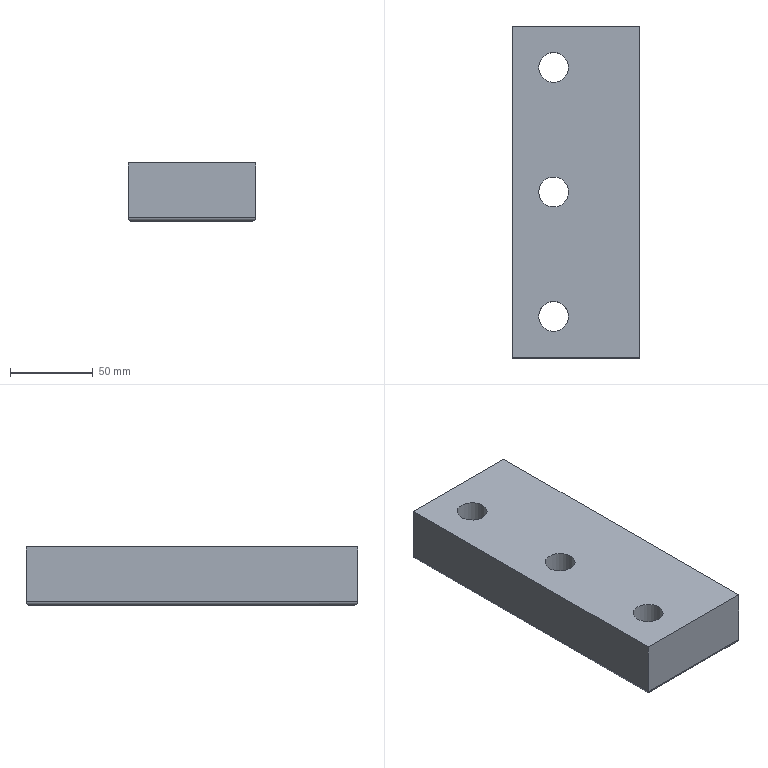Part | NX | features solid 2 | 1 solid | 13 faces | box 77 x 200 x 35 mm | volume 511808 mm3 | cylinder 7 | plane 6 | commonest cylinder face diameters 4 x4 18 x3
STEP:
#1=CARTESIAN_POINT('',(-648.,-745.,177.));
#2=VERTEX_POINT('',#1);
#3=CARTESIAN_POINT('',(-648.,-745.,210.));
#4=VERTEX_POINT('',#3);
#5=CARTESIAN_POINT('',(-648.,-745.,357.029));
#6=DIRECTION('',(0.,0.,-1.));
#7=VECTOR('',#6,1000.);
#8=LINE('',#5,#7);
#9=EDGE_CURVE('',#2,#4,#8,.F.);
#10=ORIENTED_EDGE('',*,*,#9,.F.);
#11=CARTESIAN_POINT('',(-648.,-545.,177.));
#12=VERTEX_POINT('',#11);
#13=CARTESIAN_POINT('',(-648.,-545.,177.));
#14=DIRECTION('',(0.,1.,0.));
#15=VECTOR('',#14,1000.);
#16=LINE('',#13,#15);
#17=EDGE_CURVE('',#2,#12,#16,.T.);
#18=ORIENTED_EDGE('',*,*,#17,.T.);
#19=CARTESIAN_POINT('',(-648.,-545.,210.));
#20=VERTEX_POINT('',#19);
#21=CARTESIAN_POINT('',(-648.,-545.,210.));
#22=DIRECTION('',(0.,0.,-1.));
#23=VECTOR('',#22,1000.);
#24=LINE('',#21,#23);
#25=EDGE_CURVE('',#12,#20,#24,.F.);
#26=ORIENTED_EDGE('',*,*,#25,.T.);
#27=CARTESIAN_POINT('',(-648.,-905.,210.));
#28=DIRECTION('',(0.,1.,0.));
#29=VECTOR('',#28,1000.);
#30=LINE('',#27,#29);
#31=EDGE_CURVE('',#4,#20,#30,.T.);
#32=ORIENTED_EDGE('',*,*,#31,.F.);
#33=EDGE_LOOP('',(#10,#18,#26,#32));
#34=FACE_BOUND('',#33,.T.);
#35=CARTESIAN_POINT('',(-648.,-905.,210.));
#36=DIRECTION('',(1.,0.,0.));
#37=DIRECTION('',(0.,1.,0.));
#38=AXIS2_PLACEMENT_3D('',#35,#36,#37);
#39=PLANE('',#38);
#40=ADVANCED_FACE('',(#34),#39,.T.);
#41=ORIENTED_EDGE('',*,*,#25,.F.);
#42=CARTESIAN_POINT('',(-725.,-545.,177.));
#43=VERTEX_POINT('',#42);
#44=CARTESIAN_POINT('',(-727.,-545.,177.));
#45=DIRECTION('',(-1.,0.,0.));
#46=VECTOR('',#45,1000.);
#47=LINE('',#44,#46);
#48=EDGE_CURVE('',#12,#43,#47,.T.);
#49=ORIENTED_EDGE('',*,*,#48,.T.);
#50=CARTESIAN_POINT('',(-725.,-545.,210.));
#51=VERTEX_POINT('',#50);
#52=CARTESIAN_POINT('',(-725.,-545.,268.));
#53=DIRECTION('',(0.,0.,1.));
#54=VECTOR('',#53,1000.);
#55=LINE('',#52,#54);
#56=EDGE_CURVE('',#43,#51,#55,.T.);
#57=ORIENTED_EDGE('',*,*,#56,.T.);
#58=CARTESIAN_POINT('',(-648.,-545.,210.));
#59=DIRECTION('',(1.,0.,0.));
#60=VECTOR('',#59,1000.);
#61=LINE('',#58,#60);
#62=EDGE_CURVE('',#20,#51,#61,.F.);
#63=ORIENTED_EDGE('',*,*,#62,.F.);
#64=EDGE_LOOP('',(#41,#49,#57,#63));
#65=FACE_BOUND('',#64,.T.);
#66=CARTESIAN_POINT('',(-671.,-545.,268.));
#67=DIRECTION('',(0.,-1.,0.));
#68=DIRECTION('',(1.,0.,0.));
#69=AXIS2_PLACEMENT_3D('',#66,#67,#68);
#70=PLANE('',#69);
#71=ADVANCED_FACE('',(#65),#70,.F.);
#72=ORIENTED_EDGE('',*,*,#56,.F.);
#73=CARTESIAN_POINT('',(-725.,-745.,177.));
#74=VERTEX_POINT('',#73);
#75=CARTESIAN_POINT('',(-725.,-745.,177.));
#76=DIRECTION('',(0.,1.,0.));
#77=VECTOR('',#76,1000.);
#78=LINE('',#75,#77);
#79=EDGE_CURVE('',#43,#74,#78,.F.);
#80=ORIENTED_EDGE('',*,*,#79,.T.);
#81=CARTESIAN_POINT('',(-725.,-745.,210.));
#82=VERTEX_POINT('',#81);
#83=CARTESIAN_POINT('',(-725.,-745.,210.));
#84=DIRECTION('',(0.,0.,1.));
#85=VECTOR('',#84,1000.);
#86=LINE('',#83,#85);
#87=EDGE_CURVE('',#74,#82,#86,.T.);
#88=ORIENTED_EDGE('',*,*,#87,.T.);
#89=CARTESIAN_POINT('',(-725.,-905.,210.));
#90=DIRECTION('',(0.,-1.,0.));
#91=VECTOR('',#90,1000.);
#92=LINE('',#89,#91);
#93=EDGE_CURVE('',#82,#51,#92,.F.);
#94=ORIENTED_EDGE('',*,*,#93,.T.);
#95=EDGE_LOOP('',(#72,#80,#88,#94));
#96=FACE_BOUND('',#95,.T.);
#97=CARTESIAN_POINT('',(-725.,-905.,210.));
#98=DIRECTION('',(1.,0.,0.));
#99=DIRECTION('',(0.,1.,0.));
#100=AXIS2_PLACEMENT_3D('',#97,#98,#99);
#101=PLANE('',#100);
#102=ADVANCED_FACE('',(#96),#101,.F.);
#103=ORIENTED_EDGE('',*,*,#87,.F.);
#104=CARTESIAN_POINT('',(-648.,-745.,177.));
#105=DIRECTION('',(-1.,0.,0.));
#106=VECTOR('',#105,1000.);
#107=LINE('',#104,#106);
#108=EDGE_CURVE('',#74,#2,#107,.F.);
#109=ORIENTED_EDGE('',*,*,#108,.T.);
#110=ORIENTED_EDGE('',*,*,#9,.T.);
#111=CARTESIAN_POINT('',(-71.,-745.,210.));
#112=DIRECTION('',(1.,0.,0.));
#113=VECTOR('',#112,1000.);
#114=LINE('',#111,#113);
#115=EDGE_CURVE('',#4,#82,#114,.F.);
#116=ORIENTED_EDGE('',*,*,#115,.T.);
#117=EDGE_LOOP('',(#103,#109,#110,#116));
#118=FACE_BOUND('',#117,.T.);
#119=CARTESIAN_POINT('',(-71.,-745.,357.029));
#120=DIRECTION('',(0.,1.,0.));
#121=DIRECTION('',(0.,0.,-1.));
#122=AXIS2_PLACEMENT_3D('',#119,#120,#121);
#123=PLANE('',#122);
#124=ADVANCED_FACE('',(#118),#123,.F.);
#125=CARTESIAN_POINT('',(-700.,-636.,210.));
#126=VERTEX_POINT('',#125);
#127=CARTESIAN_POINT('',(-700.,-645.,210.));
#128=DIRECTION('',(0.,0.,1.));
#129=DIRECTION('',(0.,1.,0.));
#130=AXIS2_PLACEMENT_3D('',#127,#128,#129);
#131=CIRCLE('',#130,9.);
#132=EDGE_CURVE('',#126,#126,#131,.T.);
#133=ORIENTED_EDGE('',*,*,#132,.F.);
#134=EDGE_LOOP('',(#133));
#135=FACE_BOUND('',#134,.T.);
#136=CARTESIAN_POINT('',(-700.,-561.,210.));
#137=VERTEX_POINT('',#136);
#138=CARTESIAN_POINT('',(-700.,-570.,210.));
#139=DIRECTION('',(0.,0.,1.));
#140=DIRECTION('',(0.,1.,0.));
#141=AXIS2_PLACEMENT_3D('',#138,#139,#140);
#142=CIRCLE('',#141,9.);
#143=EDGE_CURVE('',#137,#137,#142,.T.);
#144=ORIENTED_EDGE('',*,*,#143,.F.);
#145=EDGE_LOOP('',(#144));
#146=FACE_BOUND('',#145,.T.);
#147=CARTESIAN_POINT('',(-700.,-711.,210.));
#148=VERTEX_POINT('',#147);
#149=CARTESIAN_POINT('',(-700.,-720.,210.));
#150=DIRECTION('',(0.,0.,1.));
#151=DIRECTION('',(0.,1.,0.));
#152=AXIS2_PLACEMENT_3D('',#149,#150,#151);
#153=CIRCLE('',#152,9.);
#154=EDGE_CURVE('',#148,#148,#153,.T.);
#155=ORIENTED_EDGE('',*,*,#154,.F.);
#156=EDGE_LOOP('',(#155));
#157=FACE_BOUND('',#156,.T.);
#158=ORIENTED_EDGE('',*,*,#93,.F.);
#159=ORIENTED_EDGE('',*,*,#115,.F.);
#160=ORIENTED_EDGE('',*,*,#31,.T.);
#161=ORIENTED_EDGE('',*,*,#62,.T.);
#162=EDGE_LOOP('',(#158,#159,#160,#161));
#163=FACE_BOUND('',#162,.T.);
#164=CARTESIAN_POINT('',(-648.,-905.,210.));
#165=DIRECTION('',(0.,0.,1.));
#166=DIRECTION('',(0.,1.,0.));
#167=AXIS2_PLACEMENT_3D('',#164,#165,#166);
#168=PLANE('',#167);
#169=ADVANCED_FACE('',(#135,#146,#157,#163),#168,.T.);
#170=CARTESIAN_POINT('',(-650.,-743.,175.));
#171=VERTEX_POINT('',#170);
#172=CARTESIAN_POINT('',(-723.,-743.,175.));
#173=VERTEX_POINT('',#172);
#174=CARTESIAN_POINT('',(-727.,-743.,175.));
#175=DIRECTION('',(1.,0.,0.));
#176=VECTOR('',#175,1000.);
#177=LINE('',#174,#176);
#178=EDGE_CURVE('',#171,#173,#177,.F.);
#179=ORIENTED_EDGE('',*,*,#178,.T.);
#180=CARTESIAN_POINT('',(-723.,-547.,175.));
#181=VERTEX_POINT('',#180);
#182=CARTESIAN_POINT('',(-723.,-545.,175.));
#183=DIRECTION('',(0.,-1.,0.));
#184=VECTOR('',#183,1000.);
#185=LINE('',#182,#184);
#186=EDGE_CURVE('',#173,#181,#185,.F.);
#187=ORIENTED_EDGE('',*,*,#186,.T.);
#188=CARTESIAN_POINT('',(-650.,-547.,175.));
#189=VERTEX_POINT('',#188);
#190=CARTESIAN_POINT('',(-648.,-547.,175.));
#191=DIRECTION('',(1.,0.,0.));
#192=VECTOR('',#191,1000.);
#193=LINE('',#190,#192);
#194=EDGE_CURVE('',#181,#189,#193,.T.);
#195=ORIENTED_EDGE('',*,*,#194,.T.);
#196=CARTESIAN_POINT('',(-650.,-745.,175.));
#197=DIRECTION('',(0.,1.,0.));
#198=VECTOR('',#197,1000.);
#199=LINE('',#196,#198);
#200=EDGE_CURVE('',#189,#171,#199,.F.);
#201=ORIENTED_EDGE('',*,*,#200,.T.);
#202=EDGE_LOOP('',(#179,#187,#195,#201));
#203=FACE_BOUND('',#202,.T.);
#204=CARTESIAN_POINT('',(-700.,-636.,175.));
#205=VERTEX_POINT('',#204);
#206=CARTESIAN_POINT('',(-700.,-645.,175.));
#207=DIRECTION('',(0.,0.,1.));
#208=DIRECTION('',(0.,1.,0.));
#209=AXIS2_PLACEMENT_3D('',#206,#207,#208);
#210=CIRCLE('',#209,9.);
#211=EDGE_CURVE('',#205,#205,#210,.T.);
#212=ORIENTED_EDGE('',*,*,#211,.T.);
#213=EDGE_LOOP('',(#212));
#214=FACE_BOUND('',#213,.T.);
#215=CARTESIAN_POINT('',(-700.,-561.,175.));
#216=VERTEX_POINT('',#215);
#217=CARTESIAN_POINT('',(-700.,-570.,175.));
#218=DIRECTION('',(0.,0.,1.));
#219=DIRECTION('',(0.,1.,0.));
#220=AXIS2_PLACEMENT_3D('',#217,#218,#219);
#221=CIRCLE('',#220,9.);
#222=EDGE_CURVE('',#216,#216,#221,.T.);
#223=ORIENTED_EDGE('',*,*,#222,.T.);
#224=EDGE_LOOP('',(#223));
#225=FACE_BOUND('',#224,.T.);
#226=CARTESIAN_POINT('',(-700.,-711.,175.));
#227=VERTEX_POINT('',#226);
#228=CARTESIAN_POINT('',(-700.,-720.,175.));
#229=DIRECTION('',(0.,0.,1.));
#230=DIRECTION('',(0.,1.,0.));
#231=AXIS2_PLACEMENT_3D('',#228,#229,#230);
#232=CIRCLE('',#231,9.);
#233=EDGE_CURVE('',#227,#227,#232,.T.);
#234=ORIENTED_EDGE('',*,*,#233,.T.);
#235=EDGE_LOOP('',(#234));
#236=FACE_BOUND('',#235,.T.);
#237=CARTESIAN_POINT('',(-648.,-905.,175.));
#238=DIRECTION('',(0.,0.,1.));
#239=DIRECTION('',(0.,1.,0.));
#240=AXIS2_PLACEMENT_3D('',#237,#238,#239);
#241=PLANE('',#240);
#242=ADVANCED_FACE('',(#203,#214,#225,#236),#241,.F.);
#243=ORIENTED_EDGE('',*,*,#154,.T.);
#244=EDGE_LOOP('',(#243));
#245=FACE_BOUND('',#244,.T.);
#246=ORIENTED_EDGE('',*,*,#233,.F.);
#247=EDGE_LOOP('',(#246));
#248=FACE_BOUND('',#247,.T.);
#249=CARTESIAN_POINT('',(-700.,-720.,175.));
#250=DIRECTION('',(0.,0.,1.));
#251=DIRECTION('',(0.,1.,0.));
#252=AXIS2_PLACEMENT_3D('',#249,#250,#251);
#253=CYLINDRICAL_SURFACE('',#252,9.);
#254=ADVANCED_FACE('',(#245,#248),#253,.F.);
#255=ORIENTED_EDGE('',*,*,#143,.T.);
#256=EDGE_LOOP('',(#255));
#257=FACE_BOUND('',#256,.T.);
#258=ORIENTED_EDGE('',*,*,#222,.F.);
#259=EDGE_LOOP('',(#258));
#260=FACE_BOUND('',#259,.T.);
#261=CARTESIAN_POINT('',(-700.,-570.,175.));
#262=DIRECTION('',(0.,0.,1.));
#263=DIRECTION('',(0.,1.,0.));
#264=AXIS2_PLACEMENT_3D('',#261,#262,#263);
#265=CYLINDRICAL_SURFACE('',#264,9.);
#266=ADVANCED_FACE('',(#257,#260),#265,.F.);
#267=ORIENTED_EDGE('',*,*,#132,.T.);
#268=EDGE_LOOP('',(#267));
#269=FACE_BOUND('',#268,.T.);
#270=ORIENTED_EDGE('',*,*,#211,.F.);
#271=EDGE_LOOP('',(#270));
#272=FACE_BOUND('',#271,.T.);
#273=CARTESIAN_POINT('',(-700.,-645.,175.));
#274=DIRECTION('',(0.,0.,1.));
#275=DIRECTION('',(0.,1.,0.));
#276=AXIS2_PLACEMENT_3D('',#273,#274,#275);
#277=CYLINDRICAL_SURFACE('',#276,9.);
#278=ADVANCED_FACE('',(#269,#272),#277,.F.);
#279=CARTESIAN_POINT('',(-650.,-547.,177.));
#280=DIRECTION('',(0.7071,-0.7071,0.));
#281=DIRECTION('',(-0.7071,-0.7071,0.));
#282=AXIS2_PLACEMENT_3D('',#279,#280,#281);
#283=ELLIPSE('',#282,2.828,2.);
#284=EDGE_CURVE('',#12,#189,#283,.F.);
#285=ORIENTED_EDGE('',*,*,#284,.F.);
#286=ORIENTED_EDGE('',*,*,#17,.F.);
#287=CARTESIAN_POINT('',(-650.,-743.,177.));
#288=DIRECTION('',(-0.7071,-0.7071,0.));
#289=DIRECTION('',(-0.7071,0.7071,0.));
#290=AXIS2_PLACEMENT_3D('',#287,#288,#289);
#291=ELLIPSE('',#290,2.828,2.);
#292=EDGE_CURVE('',#171,#2,#291,.T.);
#293=ORIENTED_EDGE('',*,*,#292,.F.);
#294=ORIENTED_EDGE('',*,*,#200,.F.);
#295=EDGE_LOOP('',(#285,#286,#293,#294));
#296=FACE_BOUND('',#295,.T.);
#297=CARTESIAN_POINT('',(-650.,-905.,177.));
#298=DIRECTION('',(0.,-1.,0.));
#299=DIRECTION('',(0.,0.,1.));
#300=AXIS2_PLACEMENT_3D('',#297,#298,#299);
#301=CYLINDRICAL_SURFACE('',#300,2.);
#302=ADVANCED_FACE('',(#296),#301,.T.);
#303=ORIENTED_EDGE('',*,*,#292,.T.);
#304=ORIENTED_EDGE('',*,*,#108,.F.);
#305=CARTESIAN_POINT('',(-723.,-743.,177.));
#306=DIRECTION('',(-0.7071,0.7071,0.));
#307=DIRECTION('',(-0.7071,-0.7071,0.));
#308=AXIS2_PLACEMENT_3D('',#305,#306,#307);
#309=ELLIPSE('',#308,2.828,2.);
#310=EDGE_CURVE('',#173,#74,#309,.T.);
#311=ORIENTED_EDGE('',*,*,#310,.F.);
#312=ORIENTED_EDGE('',*,*,#178,.F.);
#313=EDGE_LOOP('',(#303,#304,#311,#312));
#314=FACE_BOUND('',#313,.T.);
#315=CARTESIAN_POINT('',(-648.,-743.,177.));
#316=DIRECTION('',(-1.,0.,0.));
#317=DIRECTION('',(0.,0.,1.));
#318=AXIS2_PLACEMENT_3D('',#315,#316,#317);
#319=CYLINDRICAL_SURFACE('',#318,2.);
#320=ADVANCED_FACE('',(#314),#319,.T.);
#321=ORIENTED_EDGE('',*,*,#284,.T.);
#322=ORIENTED_EDGE('',*,*,#194,.F.);
#323=CARTESIAN_POINT('',(-723.,-547.,177.));
#324=DIRECTION('',(-0.7071,-0.7071,0.));
#325=DIRECTION('',(-0.7071,0.7071,0.));
#326=AXIS2_PLACEMENT_3D('',#323,#324,#325);
#327=ELLIPSE('',#326,2.828,2.);
#328=EDGE_CURVE('',#43,#181,#327,.T.);
#329=ORIENTED_EDGE('',*,*,#328,.F.);
#330=ORIENTED_EDGE('',*,*,#48,.F.);
#331=EDGE_LOOP('',(#321,#322,#329,#330));
#332=FACE_BOUND('',#331,.T.);
#333=CARTESIAN_POINT('',(-671.,-547.,177.));
#334=DIRECTION('',(-1.,0.,0.));
#335=DIRECTION('',(0.,0.,1.));
#336=AXIS2_PLACEMENT_3D('',#333,#334,#335);
#337=CYLINDRICAL_SURFACE('',#336,2.);
#338=ADVANCED_FACE('',(#332),#337,.T.);
#339=ORIENTED_EDGE('',*,*,#310,.T.);
#340=ORIENTED_EDGE('',*,*,#79,.F.);
#341=ORIENTED_EDGE('',*,*,#328,.T.);
#342=ORIENTED_EDGE('',*,*,#186,.F.);
#343=EDGE_LOOP('',(#339,#340,#341,#342));
#344=FACE_BOUND('',#343,.T.);
#345=CARTESIAN_POINT('',(-723.,-905.,177.));
#346=DIRECTION('',(0.,1.,0.));
#347=DIRECTION('',(0.,0.,-1.));
#348=AXIS2_PLACEMENT_3D('',#345,#346,#347);
#349=CYLINDRICAL_SURFACE('',#348,2.);
#350=ADVANCED_FACE('',(#344),#349,.T.);
#351=CLOSED_SHELL('',(#40,#71,#102,#124,#169,#242,#254,#266,#278,#302,#320,#338,#350));
#352=MANIFOLD_SOLID_BREP('',#351);
#353=(LENGTH_UNIT()NAMED_UNIT(*)SI_UNIT(.MILLI.,.METRE.));
#354=UNCERTAINTY_MEASURE_WITH_UNIT(LENGTH_MEASURE(0.00001),#353,'','');
#355=(NAMED_UNIT(*)PLANE_ANGLE_UNIT()SI_UNIT($,.RADIAN.));
#356=(NAMED_UNIT(*)SI_UNIT($,.STERADIAN.)SOLID_ANGLE_UNIT());
#357=(GEOMETRIC_REPRESENTATION_CONTEXT(3)GLOBAL_UNCERTAINTY_ASSIGNED_CONTEXT((#354))GLOBAL_UNIT_ASSIGNED_CONTEXT((#353,#355,#356))REPRESENTATION_CONTEXT('',''));
#358=ADVANCED_BREP_SHAPE_REPRESENTATION('',(#352),#357);